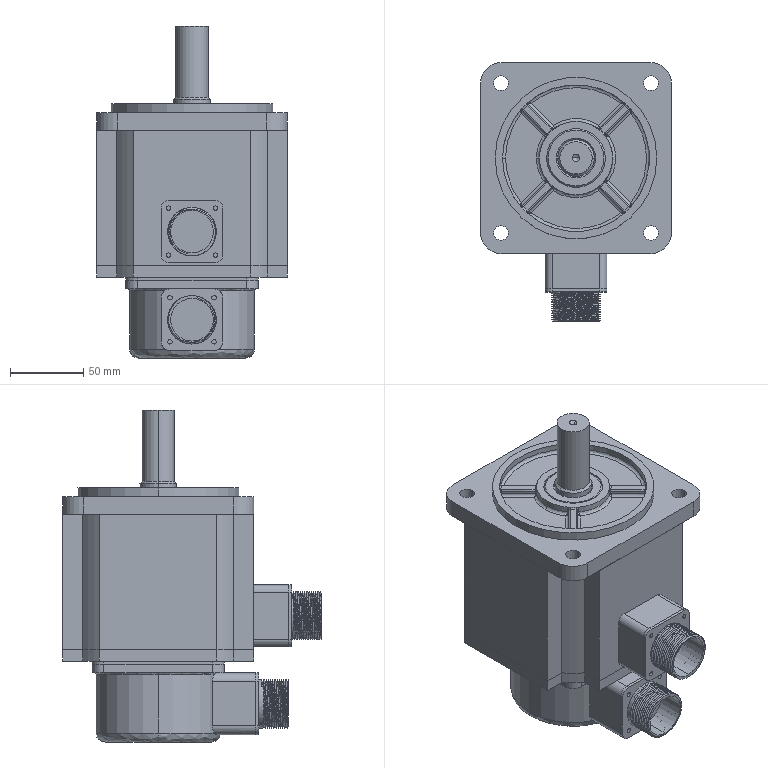Part | STEP file | 130ST-M04025LSB | 9 solids | 380 faces | box 130 x 176 x 226 mm | volume 2134855 mm3 | cylinder 210 | plane 101 | spline 61 | cone 8 | commonest cylinder face diameters 33 x55 2 x26 3 x24 4 x18 10 x16 5 x10